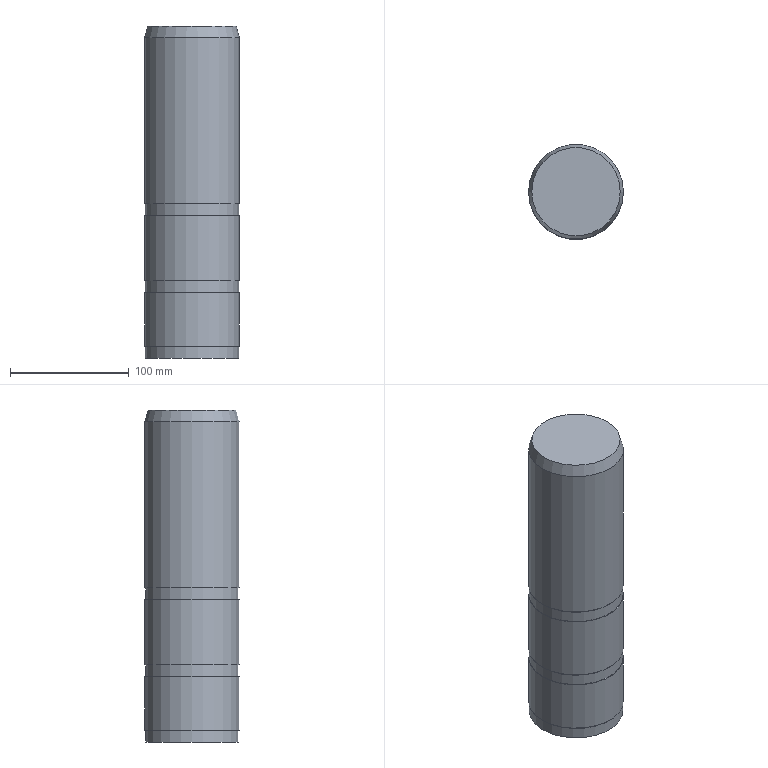Part | NX | features solid 2 | 1 solid | 14 faces | box 80 x 80 x 280 mm | volume 1400395 mm3 | plane 7 | cylinder 6 | cone 1 | commonest cylinder face diameters 79 x3 80 x3
STEP:
#1=CARTESIAN_POINT('',(1210.5,-290.,-300.));
#2=VERTEX_POINT('',#1);
#3=CARTESIAN_POINT('',(1250.,-290.,-300.));
#4=DIRECTION('',(0.,0.,1.));
#5=DIRECTION('',(-1.,0.,0.));
#6=AXIS2_PLACEMENT_3D('',#3,#4,#5);
#7=CIRCLE('',#6,39.5);
#8=EDGE_CURVE('',#2,#2,#7,.T.);
#9=ORIENTED_EDGE('',*,*,#8,.F.);
#10=EDGE_LOOP('',(#9));
#11=FACE_BOUND('',#10,.T.);
#12=CARTESIAN_POINT('',(1210.5,-290.,-310.));
#13=VERTEX_POINT('',#12);
#14=CARTESIAN_POINT('',(1250.,-290.,-310.));
#15=DIRECTION('',(0.,0.,1.));
#16=DIRECTION('',(-1.,0.,0.));
#17=AXIS2_PLACEMENT_3D('',#14,#15,#16);
#18=CIRCLE('',#17,39.5);
#19=EDGE_CURVE('',#13,#13,#18,.T.);
#20=ORIENTED_EDGE('',*,*,#19,.T.);
#21=EDGE_LOOP('',(#20));
#22=FACE_BOUND('',#21,.T.);
#23=CARTESIAN_POINT('',(1250.,-290.,-300.));
#24=DIRECTION('',(0.,0.,-1.));
#25=DIRECTION('',(1.,0.,0.));
#26=AXIS2_PLACEMENT_3D('',#23,#24,#25);
#27=CYLINDRICAL_SURFACE('',#26,39.5);
#28=ADVANCED_FACE('',(#11,#22),#27,.T.);
#29=CARTESIAN_POINT('',(1210.,-290.,-300.));
#30=VERTEX_POINT('',#29);
#31=CARTESIAN_POINT('',(1250.,-290.,-300.));
#32=DIRECTION('',(0.,0.,1.));
#33=DIRECTION('',(-1.,0.,0.));
#34=AXIS2_PLACEMENT_3D('',#31,#32,#33);
#35=CIRCLE('',#34,40.);
#36=EDGE_CURVE('',#30,#30,#35,.T.);
#37=ORIENTED_EDGE('',*,*,#36,.F.);
#38=EDGE_LOOP('',(#37));
#39=FACE_BOUND('',#38,.T.);
#40=ORIENTED_EDGE('',*,*,#8,.T.);
#41=EDGE_LOOP('',(#40));
#42=FACE_BOUND('',#41,.T.);
#43=CARTESIAN_POINT('',(1250.,-290.,-300.));
#44=DIRECTION('',(0.,0.,1.));
#45=DIRECTION('',(-1.,0.,0.));
#46=AXIS2_PLACEMENT_3D('',#43,#44,#45);
#47=PLANE('',#46);
#48=ADVANCED_FACE('',(#39,#42),#47,.F.);
#49=CARTESIAN_POINT('',(1210.,-290.,-160.));
#50=VERTEX_POINT('',#49);
#51=CARTESIAN_POINT('',(1250.,-290.,-160.));
#52=DIRECTION('',(0.,0.,1.));
#53=DIRECTION('',(-1.,0.,0.));
#54=AXIS2_PLACEMENT_3D('',#51,#52,#53);
#55=CIRCLE('',#54,40.);
#56=EDGE_CURVE('',#50,#50,#55,.T.);
#57=ORIENTED_EDGE('',*,*,#56,.F.);
#58=EDGE_LOOP('',(#57));
#59=FACE_BOUND('',#58,.T.);
#60=ORIENTED_EDGE('',*,*,#36,.T.);
#61=EDGE_LOOP('',(#60));
#62=FACE_BOUND('',#61,.T.);
#63=CARTESIAN_POINT('',(1250.,-290.,-140.));
#64=DIRECTION('',(0.,0.,-1.));
#65=DIRECTION('',(1.,0.,0.));
#66=AXIS2_PLACEMENT_3D('',#63,#64,#65);
#67=CYLINDRICAL_SURFACE('',#66,40.);
#68=ADVANCED_FACE('',(#59,#62),#67,.T.);
#69=CARTESIAN_POINT('',(1212.679,-290.,-150.));
#70=VERTEX_POINT('',#69);
#71=CARTESIAN_POINT('',(1250.,-290.,-150.));
#72=DIRECTION('',(0.,0.,1.));
#73=DIRECTION('',(-1.,0.,0.));
#74=AXIS2_PLACEMENT_3D('',#71,#72,#73);
#75=CIRCLE('',#74,37.321);
#76=EDGE_CURVE('',#70,#70,#75,.T.);
#77=ORIENTED_EDGE('',*,*,#76,.F.);
#78=EDGE_LOOP('',(#77));
#79=FACE_BOUND('',#78,.T.);
#80=ORIENTED_EDGE('',*,*,#56,.T.);
#81=EDGE_LOOP('',(#80));
#82=FACE_BOUND('',#81,.T.);
#83=CARTESIAN_POINT('',(1250.,-290.,-160.));
#84=DIRECTION('',(0.,0.,-1.));
#85=DIRECTION('',(-1.,0.,0.));
#86=AXIS2_PLACEMENT_3D('',#83,#84,#85);
#87=CONICAL_SURFACE('',#86,40.,0.2618);
#88=ADVANCED_FACE('',(#79,#82),#87,.T.);
#89=ORIENTED_EDGE('',*,*,#76,.T.);
#90=EDGE_LOOP('',(#89));
#91=FACE_BOUND('',#90,.T.);
#92=CARTESIAN_POINT('',(1250.,-290.,-150.));
#93=DIRECTION('',(0.,0.,1.));
#94=DIRECTION('',(-1.,0.,0.));
#95=AXIS2_PLACEMENT_3D('',#92,#93,#94);
#96=PLANE('',#95);
#97=ADVANCED_FACE('',(#91),#96,.T.);
#98=CARTESIAN_POINT('',(1210.,-290.,-310.));
#99=VERTEX_POINT('',#98);
#100=CARTESIAN_POINT('',(1250.,-290.,-310.));
#101=DIRECTION('',(0.,0.,1.));
#102=DIRECTION('',(-1.,0.,0.));
#103=AXIS2_PLACEMENT_3D('',#100,#101,#102);
#104=CIRCLE('',#103,40.);
#105=EDGE_CURVE('',#99,#99,#104,.T.);
#106=ORIENTED_EDGE('',*,*,#105,.T.);
#107=EDGE_LOOP('',(#106));
#108=FACE_BOUND('',#107,.T.);
#109=ORIENTED_EDGE('',*,*,#19,.F.);
#110=EDGE_LOOP('',(#109));
#111=FACE_BOUND('',#110,.T.);
#112=CARTESIAN_POINT('',(1250.,-290.,-310.));
#113=DIRECTION('',(0.,0.,1.));
#114=DIRECTION('',(-1.,0.,0.));
#115=AXIS2_PLACEMENT_3D('',#112,#113,#114);
#116=PLANE('',#115);
#117=ADVANCED_FACE('',(#108,#111),#116,.T.);
#118=CARTESIAN_POINT('',(1210.,-290.,-365.));
#119=VERTEX_POINT('',#118);
#120=CARTESIAN_POINT('',(1250.,-290.,-365.));
#121=DIRECTION('',(0.,0.,1.));
#122=DIRECTION('',(-1.,0.,0.));
#123=AXIS2_PLACEMENT_3D('',#120,#121,#122);
#124=CIRCLE('',#123,40.);
#125=EDGE_CURVE('',#119,#119,#124,.T.);
#126=ORIENTED_EDGE('',*,*,#125,.T.);
#127=EDGE_LOOP('',(#126));
#128=FACE_BOUND('',#127,.T.);
#129=ORIENTED_EDGE('',*,*,#105,.F.);
#130=EDGE_LOOP('',(#129));
#131=FACE_BOUND('',#130,.T.);
#132=CARTESIAN_POINT('',(1250.,-290.,-365.));
#133=DIRECTION('',(0.,0.,1.));
#134=DIRECTION('',(-1.,0.,0.));
#135=AXIS2_PLACEMENT_3D('',#132,#133,#134);
#136=CYLINDRICAL_SURFACE('',#135,40.);
#137=ADVANCED_FACE('',(#128,#131),#136,.T.);
#138=CARTESIAN_POINT('',(1210.5,-290.,-365.));
#139=VERTEX_POINT('',#138);
#140=CARTESIAN_POINT('',(1250.,-290.,-365.));
#141=DIRECTION('',(0.,0.,1.));
#142=DIRECTION('',(-1.,0.,0.));
#143=AXIS2_PLACEMENT_3D('',#140,#141,#142);
#144=CIRCLE('',#143,39.5);
#145=EDGE_CURVE('',#139,#139,#144,.T.);
#146=ORIENTED_EDGE('',*,*,#145,.T.);
#147=EDGE_LOOP('',(#146));
#148=FACE_BOUND('',#147,.T.);
#149=ORIENTED_EDGE('',*,*,#125,.F.);
#150=EDGE_LOOP('',(#149));
#151=FACE_BOUND('',#150,.T.);
#152=CARTESIAN_POINT('',(1250.,-290.,-365.));
#153=DIRECTION('',(0.,0.,1.));
#154=DIRECTION('',(-1.,0.,0.));
#155=AXIS2_PLACEMENT_3D('',#152,#153,#154);
#156=PLANE('',#155);
#157=ADVANCED_FACE('',(#148,#151),#156,.F.);
#158=CARTESIAN_POINT('',(1210.5,-290.,-375.));
#159=VERTEX_POINT('',#158);
#160=CARTESIAN_POINT('',(1250.,-290.,-375.));
#161=DIRECTION('',(0.,0.,1.));
#162=DIRECTION('',(-1.,0.,0.));
#163=AXIS2_PLACEMENT_3D('',#160,#161,#162);
#164=CIRCLE('',#163,39.5);
#165=EDGE_CURVE('',#159,#159,#164,.F.);
#166=ORIENTED_EDGE('',*,*,#165,.F.);
#167=EDGE_LOOP('',(#166));
#168=FACE_BOUND('',#167,.T.);
#169=ORIENTED_EDGE('',*,*,#145,.F.);
#170=EDGE_LOOP('',(#169));
#171=FACE_BOUND('',#170,.T.);
#172=CARTESIAN_POINT('',(1250.,-290.,-375.));
#173=DIRECTION('',(0.,0.,1.));
#174=DIRECTION('',(-1.,0.,0.));
#175=AXIS2_PLACEMENT_3D('',#172,#173,#174);
#176=CYLINDRICAL_SURFACE('',#175,39.5);
#177=ADVANCED_FACE('',(#168,#171),#176,.T.);
#178=CARTESIAN_POINT('',(1210.,-290.,-420.));
#179=VERTEX_POINT('',#178);
#180=CARTESIAN_POINT('',(1250.,-290.,-420.));
#181=DIRECTION('',(0.,0.,1.));
#182=DIRECTION('',(-1.,0.,0.));
#183=AXIS2_PLACEMENT_3D('',#180,#181,#182);
#184=CIRCLE('',#183,40.);
#185=EDGE_CURVE('',#179,#179,#184,.T.);
#186=ORIENTED_EDGE('',*,*,#185,.T.);
#187=EDGE_LOOP('',(#186));
#188=FACE_BOUND('',#187,.T.);
#189=CARTESIAN_POINT('',(1210.,-290.,-375.));
#190=VERTEX_POINT('',#189);
#191=CARTESIAN_POINT('',(1250.,-290.,-375.));
#192=DIRECTION('',(0.,0.,1.));
#193=DIRECTION('',(-1.,0.,0.));
#194=AXIS2_PLACEMENT_3D('',#191,#192,#193);
#195=CIRCLE('',#194,40.);
#196=EDGE_CURVE('',#190,#190,#195,.T.);
#197=ORIENTED_EDGE('',*,*,#196,.F.);
#198=EDGE_LOOP('',(#197));
#199=FACE_BOUND('',#198,.T.);
#200=CARTESIAN_POINT('',(1250.,-290.,-420.));
#201=DIRECTION('',(0.,0.,1.));
#202=DIRECTION('',(-1.,0.,0.));
#203=AXIS2_PLACEMENT_3D('',#200,#201,#202);
#204=CYLINDRICAL_SURFACE('',#203,40.);
#205=ADVANCED_FACE('',(#188,#199),#204,.T.);
#206=CARTESIAN_POINT('',(1210.5,-290.,-420.));
#207=VERTEX_POINT('',#206);
#208=CARTESIAN_POINT('',(1250.,-290.,-420.));
#209=DIRECTION('',(0.,0.,1.));
#210=DIRECTION('',(-1.,0.,0.));
#211=AXIS2_PLACEMENT_3D('',#208,#209,#210);
#212=CIRCLE('',#211,39.5);
#213=EDGE_CURVE('',#207,#207,#212,.T.);
#214=ORIENTED_EDGE('',*,*,#213,.T.);
#215=EDGE_LOOP('',(#214));
#216=FACE_BOUND('',#215,.T.);
#217=ORIENTED_EDGE('',*,*,#185,.F.);
#218=EDGE_LOOP('',(#217));
#219=FACE_BOUND('',#218,.T.);
#220=CARTESIAN_POINT('',(1250.,-290.,-420.));
#221=DIRECTION('',(0.,0.,1.));
#222=DIRECTION('',(-1.,0.,0.));
#223=AXIS2_PLACEMENT_3D('',#220,#221,#222);
#224=PLANE('',#223);
#225=ADVANCED_FACE('',(#216,#219),#224,.F.);
#226=ORIENTED_EDGE('',*,*,#165,.T.);
#227=EDGE_LOOP('',(#226));
#228=FACE_BOUND('',#227,.T.);
#229=ORIENTED_EDGE('',*,*,#196,.T.);
#230=EDGE_LOOP('',(#229));
#231=FACE_BOUND('',#230,.T.);
#232=CARTESIAN_POINT('',(1250.,-290.,-375.));
#233=DIRECTION('',(0.,0.,1.));
#234=DIRECTION('',(-1.,0.,0.));
#235=AXIS2_PLACEMENT_3D('',#232,#233,#234);
#236=PLANE('',#235);
#237=ADVANCED_FACE('',(#228,#231),#236,.T.);
#238=CARTESIAN_POINT('',(1210.5,-290.,-430.));
#239=VERTEX_POINT('',#238);
#240=CARTESIAN_POINT('',(1250.,-290.,-430.));
#241=DIRECTION('',(0.,0.,1.));
#242=DIRECTION('',(-1.,0.,0.));
#243=AXIS2_PLACEMENT_3D('',#240,#241,#242);
#244=CIRCLE('',#243,39.5);
#245=EDGE_CURVE('',#239,#239,#244,.T.);
#246=ORIENTED_EDGE('',*,*,#245,.T.);
#247=EDGE_LOOP('',(#246));
#248=FACE_BOUND('',#247,.T.);
#249=ORIENTED_EDGE('',*,*,#213,.F.);
#250=EDGE_LOOP('',(#249));
#251=FACE_BOUND('',#250,.T.);
#252=CARTESIAN_POINT('',(1250.,-290.,-430.));
#253=DIRECTION('',(0.,0.,1.));
#254=DIRECTION('',(-1.,0.,0.));
#255=AXIS2_PLACEMENT_3D('',#252,#253,#254);
#256=CYLINDRICAL_SURFACE('',#255,39.5);
#257=ADVANCED_FACE('',(#248,#251),#256,.T.);
#258=ORIENTED_EDGE('',*,*,#245,.F.);
#259=EDGE_LOOP('',(#258));
#260=FACE_BOUND('',#259,.T.);
#261=CARTESIAN_POINT('',(1250.,-290.,-430.));
#262=DIRECTION('',(0.,0.,1.));
#263=DIRECTION('',(-1.,0.,0.));
#264=AXIS2_PLACEMENT_3D('',#261,#262,#263);
#265=PLANE('',#264);
#266=ADVANCED_FACE('',(#260),#265,.F.);
#267=CLOSED_SHELL('',(#28,#48,#68,#88,#97,#117,#137,#157,#177,#205,#225,#237,#257,#266));
#268=MANIFOLD_SOLID_BREP('',#267);
#269=(LENGTH_UNIT()NAMED_UNIT(*)SI_UNIT(.MILLI.,.METRE.));
#270=UNCERTAINTY_MEASURE_WITH_UNIT(LENGTH_MEASURE(0.00001),#269,'','');
#271=(NAMED_UNIT(*)PLANE_ANGLE_UNIT()SI_UNIT($,.RADIAN.));
#272=(NAMED_UNIT(*)SI_UNIT($,.STERADIAN.)SOLID_ANGLE_UNIT());
#273=(GEOMETRIC_REPRESENTATION_CONTEXT(3)GLOBAL_UNCERTAINTY_ASSIGNED_CONTEXT((#270))GLOBAL_UNIT_ASSIGNED_CONTEXT((#269,#271,#272))REPRESENTATION_CONTEXT('',''));
#274=ADVANCED_BREP_SHAPE_REPRESENTATION('',(#268),#273);